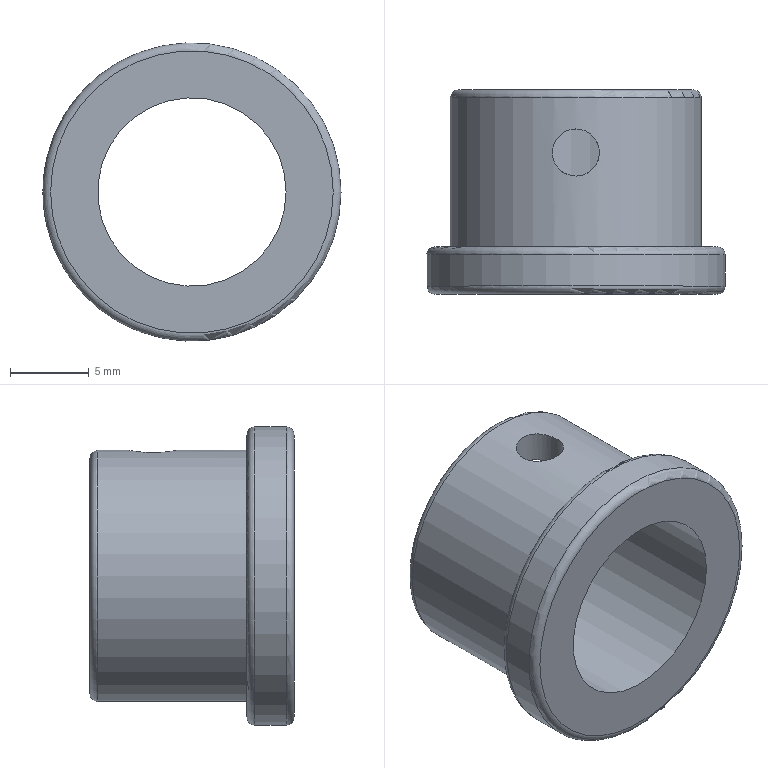Part | STEP file | 1-04.4 | 1 solid | 10 faces | box 19 x 13 x 19 mm | volume 1368 mm3 | cylinder 4 | plane 3 | torus 3 | commonest cylinder face diameters 3 x1 12 x1 16 x1 19 x1
STEP:
#1=CARTESIAN_POINT('',(0.,0.,0.));
#2=DIRECTION('',(0.,0.,1.));
#3=DIRECTION('',(1.,0.,0.));
#4=AXIS2_PLACEMENT_3D('',#1,#2,#3);
#5=CARTESIAN_POINT('',(6.,-3.,0.));
#6=VERTEX_POINT('',#5);
#7=CARTESIAN_POINT('',(6.,10.,0.));
#8=VERTEX_POINT('',#7);
#9=CARTESIAN_POINT('',(6.,-3.,0.));
#10=DIRECTION('',(0.,1.,0.));
#11=VECTOR('',#10,1.);
#12=LINE('',#9,#11);
#13=CARTESIAN_POINT('',(0.,-3.,0.));
#14=DIRECTION('',(0.,1.,0.));
#15=DIRECTION('',(1.,0.,0.));
#16=AXIS2_PLACEMENT_3D('',#13,#14,#15);
#17=CYLINDRICAL_SURFACE('',#16,6.);
#18=CARTESIAN_POINT('',(6.283,0.));
#19=DIRECTION('',(0.,1.));
#20=VECTOR('',#19,1.);
#21=LINE('',#18,#20);
#22=(GEOMETRIC_REPRESENTATION_CONTEXT(2)PARAMETRIC_REPRESENTATION_CONTEXT()REPRESENTATION_CONTEXT('',''));
#23=DEFINITIONAL_REPRESENTATION('',(#21),#22);
#24=PCURVE('',#17,#23);
#25=CARTESIAN_POINT('',(0.,0.));
#26=DIRECTION('',(0.,1.));
#27=VECTOR('',#26,1.);
#28=LINE('',#25,#27);
#29=(GEOMETRIC_REPRESENTATION_CONTEXT(2)PARAMETRIC_REPRESENTATION_CONTEXT()REPRESENTATION_CONTEXT('',''));
#30=DEFINITIONAL_REPRESENTATION('',(#28),#29);
#31=PCURVE('',#17,#30);
#32=SEAM_CURVE('',#12,(#24,#31),.PCURVE_S1.);
#33=EDGE_CURVE('',#6,#8,#32,.T.);
#34=ORIENTED_EDGE('',*,*,#33,.T.);
#35=CARTESIAN_POINT('',(0.,10.,0.));
#36=DIRECTION('',(0.,-1.,0.));
#37=DIRECTION('',(1.,0.,0.));
#38=AXIS2_PLACEMENT_3D('',#35,#36,#37);
#39=CIRCLE('',#38,6.);
#40=CARTESIAN_POINT('',(6.283,13.));
#41=DIRECTION('',(-1.,0.));
#42=VECTOR('',#41,1.);
#43=LINE('',#40,#42);
#44=(GEOMETRIC_REPRESENTATION_CONTEXT(2)PARAMETRIC_REPRESENTATION_CONTEXT()REPRESENTATION_CONTEXT('',''));
#45=DEFINITIONAL_REPRESENTATION('',(#43),#44);
#46=PCURVE('',#17,#45);
#47=CARTESIAN_POINT('',(-2.144,10.,0.));
#48=DIRECTION('',(0.,-1.,0.));
#49=DIRECTION('',(1.,0.,0.));
#50=AXIS2_PLACEMENT_3D('',#47,#48,#49);
#51=PLANE('',#50);
#52=CARTESIAN_POINT('',(2.144,0.));
#53=DIRECTION('',(1.,0.));
#54=AXIS2_PLACEMENT_2D('',#52,#53);
#55=CIRCLE('',#54,6.);
#56=(GEOMETRIC_REPRESENTATION_CONTEXT(2)PARAMETRIC_REPRESENTATION_CONTEXT()REPRESENTATION_CONTEXT('',''));
#57=DEFINITIONAL_REPRESENTATION('',(#55),#56);
#58=PCURVE('',#51,#57);
#59=SURFACE_CURVE('',#39,(#46,#58),.PCURVE_S1.);
#60=EDGE_CURVE('',#8,#8,#59,.T.);
#61=ORIENTED_EDGE('',*,*,#60,.T.);
#62=ORIENTED_EDGE('',*,*,#33,.F.);
#63=CARTESIAN_POINT('',(0.,-3.,0.));
#64=DIRECTION('',(0.,-1.,0.));
#65=DIRECTION('',(1.,0.,0.));
#66=AXIS2_PLACEMENT_3D('',#63,#64,#65);
#67=CIRCLE('',#66,6.);
#68=CARTESIAN_POINT('',(6.283,0.));
#69=DIRECTION('',(-1.,0.));
#70=VECTOR('',#69,1.);
#71=LINE('',#68,#70);
#72=(GEOMETRIC_REPRESENTATION_CONTEXT(2)PARAMETRIC_REPRESENTATION_CONTEXT()REPRESENTATION_CONTEXT('',''));
#73=DEFINITIONAL_REPRESENTATION('',(#71),#72);
#74=PCURVE('',#17,#73);
#75=CARTESIAN_POINT('',(-2.546,-3.,0.));
#76=DIRECTION('',(0.,-1.,0.));
#77=DIRECTION('',(1.,0.,0.));
#78=AXIS2_PLACEMENT_3D('',#75,#76,#77);
#79=PLANE('',#78);
#80=CARTESIAN_POINT('',(2.546,0.));
#81=DIRECTION('',(1.,0.));
#82=AXIS2_PLACEMENT_2D('',#80,#81);
#83=CIRCLE('',#82,6.);
#84=(GEOMETRIC_REPRESENTATION_CONTEXT(2)PARAMETRIC_REPRESENTATION_CONTEXT()REPRESENTATION_CONTEXT('',''));
#85=DEFINITIONAL_REPRESENTATION('',(#83),#84);
#86=PCURVE('',#79,#85);
#87=SURFACE_CURVE('',#67,(#74,#86),.PCURVE_S1.);
#88=EDGE_CURVE('',#6,#6,#87,.T.);
#89=ORIENTED_EDGE('',*,*,#88,.F.);
#90=EDGE_LOOP('',(#34,#61,#62,#89));
#91=FACE_BOUND('',#90,.F.);
#92=CARTESIAN_POINT('',(0.,7.5,6.));
#93=VERTEX_POINT('',#92);
#94=CARTESIAN_POINT('',(0.,7.5,6.));
#95=CARTESIAN_POINT('',(0.2261,7.5,6.));
#96=CARTESIAN_POINT('',(0.9044,7.347,5.962));
#97=CARTESIAN_POINT('',(1.361,6.771,5.844));
#98=CARTESIAN_POINT('',(1.591,5.777,5.787));
#99=CARTESIAN_POINT('',(1.391,5.199,5.854));
#100=CARTESIAN_POINT('',(0.5075,4.478,5.995));
#101=CARTESIAN_POINT('',(-0.09537,4.397,6.022));
#102=CARTESIAN_POINT('',(-1.153,4.875,5.913));
#103=CARTESIAN_POINT('',(-1.5,5.408,5.809));
#104=CARTESIAN_POINT('',(-1.5,6.74,5.809));
#105=CARTESIAN_POINT('',(-0.9622,7.368,5.967));
#106=CARTESIAN_POINT('',(-0.18,7.49,5.998));
#107=CARTESIAN_POINT('',(-0.1029,7.498,6.));
#108=CARTESIAN_POINT('',(-0.02572,7.5,6.));
#109=CARTESIAN_POINT('',(0.,7.5,6.));
#110=B_SPLINE_CURVE_WITH_KNOTS('',3,(#94,#95,#96,#97,#98,#99,#100,#101,#102,#103,#104,#105,#106,#107,#108,#109),.UNSPECIFIED.,.T.,.F.,(1,3,1,2,2,2,2,2,1,3,1),(-0.03834,0.,0.3333,1.,1.864,2.726,3.611,4.715,4.792,4.83,5.163),.UNSPECIFIED.);
#111=CARTESIAN_POINT('',(4.712,10.5));
#112=CARTESIAN_POINT('',(4.725,10.5));
#113=CARTESIAN_POINT('',(4.75,10.489));
#114=CARTESIAN_POINT('',(4.786,10.44));
#115=CARTESIAN_POINT('',(4.821,10.359));
#116=CARTESIAN_POINT('',(4.853,10.248));
#117=CARTESIAN_POINT('',(4.882,10.11));
#118=CARTESIAN_POINT('',(4.908,9.949));
#119=CARTESIAN_POINT('',(4.929,9.768));
#120=CARTESIAN_POINT('',(4.946,9.572));
#121=CARTESIAN_POINT('',(4.958,9.362));
#122=CARTESIAN_POINT('',(4.965,9.147));
#123=CARTESIAN_POINT('',(4.966,8.934));
#124=CARTESIAN_POINT('',(4.961,8.724));
#125=CARTESIAN_POINT('',(4.952,8.52));
#126=CARTESIAN_POINT('',(4.939,8.327));
#127=CARTESIAN_POINT('',(4.92,8.145));
#128=CARTESIAN_POINT('',(4.898,7.98));
#129=CARTESIAN_POINT('',(4.871,7.831));
#130=CARTESIAN_POINT('',(4.841,7.707));
#131=CARTESIAN_POINT('',(4.81,7.612));
#132=CARTESIAN_POINT('',(4.776,7.544));
#133=CARTESIAN_POINT('',(4.742,7.505));
#134=CARTESIAN_POINT('',(4.707,7.495));
#135=CARTESIAN_POINT('',(4.672,7.514));
#136=CARTESIAN_POINT('',(4.638,7.563));
#137=CARTESIAN_POINT('',(4.603,7.643));
#138=CARTESIAN_POINT('',(4.572,7.751));
#139=CARTESIAN_POINT('',(4.544,7.883));
#140=CARTESIAN_POINT('',(4.519,8.035));
#141=CARTESIAN_POINT('',(4.498,8.207));
#142=CARTESIAN_POINT('',(4.481,8.394));
#143=CARTESIAN_POINT('',(4.468,8.594));
#144=CARTESIAN_POINT('',(4.461,8.804));
#145=CARTESIAN_POINT('',(4.459,9.024));
#146=CARTESIAN_POINT('',(4.462,9.241));
#147=CARTESIAN_POINT('',(4.471,9.448));
#148=CARTESIAN_POINT('',(4.484,9.644));
#149=CARTESIAN_POINT('',(4.501,9.826));
#150=CARTESIAN_POINT('',(4.523,9.991));
#151=CARTESIAN_POINT('',(4.547,10.138));
#152=CARTESIAN_POINT('',(4.576,10.263));
#153=CARTESIAN_POINT('',(4.606,10.365));
#154=CARTESIAN_POINT('',(4.64,10.441));
#155=CARTESIAN_POINT('',(4.675,10.489));
#156=CARTESIAN_POINT('',(4.7,10.5));
#157=CARTESIAN_POINT('',(4.712,10.5));
#158=B_SPLINE_CURVE_WITH_KNOTS('',3,(#111,#112,#113,#114,#115,#116,#117,#118,#119,#120,#121,#122,#123,#124,#125,#126,#127,#128,#129,#130,#131,#132,#133,#134,#135,#136,#137,#138,#139,#140,#141,#142,#143,#144,#145,#146,#147,#148,#149,#150,#151,#152,#153,#154,#155,#156,#157),.UNSPECIFIED.,.T.,.F.,(4,1,1,1,1,1,1,1,1,1,1,1,1,1,1,1,1,1,1,1,1,1,1,1,1,1,1,1,1,1,1,1,1,1,1,1,1,1,1,1,1,1,1,1,4),(0.,0.1098,0.2195,0.3293,0.4391,0.5489,0.6586,0.7684,0.8782,0.9879,1.098,1.207,1.317,1.427,1.537,1.647,1.756,1.866,1.976,2.086,2.195,2.305,2.415,2.525,2.634,2.744,2.854,2.964,3.074,3.183,3.293,3.403,3.513,3.622,3.732,3.842,3.952,4.062,4.171,4.281,4.391,4.501,4.61,4.72,4.83),.QUASI_UNIFORM_KNOTS.);
#159=(GEOMETRIC_REPRESENTATION_CONTEXT(2)PARAMETRIC_REPRESENTATION_CONTEXT()REPRESENTATION_CONTEXT('',''));
#160=DEFINITIONAL_REPRESENTATION('',(#158),#159);
#161=PCURVE('',#17,#160);
#162=CARTESIAN_POINT('',(0.,6.,0.));
#163=DIRECTION('',(0.,0.,1.));
#164=DIRECTION('',(0.,1.,0.));
#165=AXIS2_PLACEMENT_3D('',#162,#163,#164);
#166=CYLINDRICAL_SURFACE('',#165,1.5);
#167=CARTESIAN_POINT('',(6.283,6.));
#168=CARTESIAN_POINT('',(6.234,6.));
#169=CARTESIAN_POINT('',(6.134,5.997));
#170=CARTESIAN_POINT('',(5.986,5.986));
#171=CARTESIAN_POINT('',(5.838,5.967));
#172=CARTESIAN_POINT('',(5.691,5.943));
#173=CARTESIAN_POINT('',(5.543,5.916));
#174=CARTESIAN_POINT('',(5.396,5.888));
#175=CARTESIAN_POINT('',(5.249,5.86));
#176=CARTESIAN_POINT('',(5.102,5.837));
#177=CARTESIAN_POINT('',(4.956,5.819));
#178=CARTESIAN_POINT('',(4.81,5.81));
#179=CARTESIAN_POINT('',(4.668,5.811));
#180=CARTESIAN_POINT('',(4.528,5.818));
#181=CARTESIAN_POINT('',(4.388,5.832));
#182=CARTESIAN_POINT('',(4.249,5.85));
#183=CARTESIAN_POINT('',(4.109,5.873));
#184=CARTESIAN_POINT('',(3.968,5.898));
#185=CARTESIAN_POINT('',(3.823,5.925));
#186=CARTESIAN_POINT('',(3.68,5.951));
#187=CARTESIAN_POINT('',(3.539,5.971));
#188=CARTESIAN_POINT('',(3.399,5.985));
#189=CARTESIAN_POINT('',(3.26,5.995));
#190=CARTESIAN_POINT('',(3.121,5.998));
#191=CARTESIAN_POINT('',(2.98,5.994));
#192=CARTESIAN_POINT('',(2.839,5.984));
#193=CARTESIAN_POINT('',(2.693,5.966));
#194=CARTESIAN_POINT('',(2.549,5.942));
#195=CARTESIAN_POINT('',(2.407,5.916));
#196=CARTESIAN_POINT('',(2.266,5.89));
#197=CARTESIAN_POINT('',(2.126,5.864));
#198=CARTESIAN_POINT('',(1.986,5.842));
#199=CARTESIAN_POINT('',(1.844,5.824));
#200=CARTESIAN_POINT('',(1.701,5.812));
#201=CARTESIAN_POINT('',(1.555,5.808));
#202=CARTESIAN_POINT('',(1.41,5.814));
#203=CARTESIAN_POINT('',(1.268,5.827));
#204=CARTESIAN_POINT('',(1.129,5.846));
#205=CARTESIAN_POINT('',(0.9901,5.868));
#206=CARTESIAN_POINT('',(0.852,5.894));
#207=CARTESIAN_POINT('',(0.7139,5.92));
#208=CARTESIAN_POINT('',(0.5752,5.945));
#209=CARTESIAN_POINT('',(0.4353,5.967));
#210=CARTESIAN_POINT('',(0.2934,5.985));
#211=CARTESIAN_POINT('',(0.1477,5.997));
#212=CARTESIAN_POINT('',(0.04935,6.));
#213=CARTESIAN_POINT('',(0.,6.));
#214=B_SPLINE_CURVE_WITH_KNOTS('',3,(#167,#168,#169,#170,#171,#172,#173,#174,#175,#176,#177,#178,#179,#180,#181,#182,#183,#184,#185,#186,#187,#188,#189,#190,#191,#192,#193,#194,#195,#196,#197,#198,#199,#200,#201,#202,#203,#204,#205,#206,#207,#208,#209,#210,#211,#212,#213),.UNSPECIFIED.,.F.,.F.,(4,1,1,1,1,1,1,1,1,1,1,1,1,1,1,1,1,1,1,1,1,1,1,1,1,1,1,1,1,1,1,1,1,1,1,1,1,1,1,1,1,1,1,1,4),(0.,0.1098,0.2195,0.3293,0.4391,0.5489,0.6586,0.7684,0.8782,0.9879,1.098,1.207,1.317,1.427,1.537,1.647,1.756,1.866,1.976,2.086,2.195,2.305,2.415,2.525,2.634,2.744,2.854,2.964,3.074,3.183,3.293,3.403,3.513,3.622,3.732,3.842,3.952,4.062,4.171,4.281,4.391,4.501,4.61,4.72,4.83),.QUASI_UNIFORM_KNOTS.);
#215=(GEOMETRIC_REPRESENTATION_CONTEXT(2)PARAMETRIC_REPRESENTATION_CONTEXT()REPRESENTATION_CONTEXT('',''));
#216=DEFINITIONAL_REPRESENTATION('',(#214),#215);
#217=PCURVE('',#166,#216);
#218=SURFACE_CURVE('',#110,(#161,#217),.PCURVE_S1.);
#219=EDGE_CURVE('',#93,#93,#218,.T.);
#220=ORIENTED_EDGE('',*,*,#219,.T.);
#221=EDGE_LOOP('',(#220));
#222=FACE_BOUND('',#221,.F.);
#223=ADVANCED_FACE('',(#91,#222),#17,.F.);
#224=CARTESIAN_POINT('',(0.,7.5,8.));
#225=VERTEX_POINT('',#224);
#226=CARTESIAN_POINT('',(0.,7.5,6.));
#227=DIRECTION('',(0.,0.,1.));
#228=VECTOR('',#227,1.);
#229=LINE('',#226,#228);
#230=CARTESIAN_POINT('',(0.,6.));
#231=DIRECTION('',(0.,1.));
#232=VECTOR('',#231,1.);
#233=LINE('',#230,#232);
#234=(GEOMETRIC_REPRESENTATION_CONTEXT(2)PARAMETRIC_REPRESENTATION_CONTEXT()REPRESENTATION_CONTEXT('',''));
#235=DEFINITIONAL_REPRESENTATION('',(#233),#234);
#236=PCURVE('',#166,#235);
#237=CARTESIAN_POINT('',(6.283,6.));
#238=DIRECTION('',(0.,1.));
#239=VECTOR('',#238,1.);
#240=LINE('',#237,#239);
#241=(GEOMETRIC_REPRESENTATION_CONTEXT(2)PARAMETRIC_REPRESENTATION_CONTEXT()REPRESENTATION_CONTEXT('',''));
#242=DEFINITIONAL_REPRESENTATION('',(#240),#241);
#243=PCURVE('',#166,#242);
#244=SEAM_CURVE('',#229,(#236,#243),.PCURVE_S1.);
#245=EDGE_CURVE('',#93,#225,#244,.T.);
#246=ORIENTED_EDGE('',*,*,#245,.F.);
#247=ORIENTED_EDGE('',*,*,#219,.F.);
#248=ORIENTED_EDGE('',*,*,#245,.T.);
#249=CARTESIAN_POINT('',(0.,7.5,8.));
#250=CARTESIAN_POINT('',(-0.03438,7.5,8.));
#251=CARTESIAN_POINT('',(-0.1375,7.496,7.999));
#252=CARTESIAN_POINT('',(-0.2404,7.482,7.997));
#253=CARTESIAN_POINT('',(-1.002,7.323,7.967));
#254=CARTESIAN_POINT('',(-1.5,6.712,7.858));
#255=CARTESIAN_POINT('',(-1.5,5.288,7.858));
#256=CARTESIAN_POINT('',(-1.002,4.677,7.967));
#257=CARTESIAN_POINT('',(0.7679,4.306,8.035));
#258=CARTESIAN_POINT('',(1.71,5.272,7.819));
#259=CARTESIAN_POINT('',(1.36,6.774,7.884));
#260=CARTESIAN_POINT('',(0.9023,7.347,7.971));
#261=CARTESIAN_POINT('',(0.2256,7.5,8.));
#262=CARTESIAN_POINT('',(0.,7.5,8.));
#263=B_SPLINE_CURVE_WITH_KNOTS('',3,(#249,#250,#251,#252,#253,#254,#255,#256,#257,#258,#259,#260,#261,#262),.UNSPECIFIED.,.T.,.F.,(1,3,1,2,2,2,2,1,3,1),(-0.3333,0.,0.05142,0.1542,1.216,2.277,3.922,4.589,4.922,4.974),.UNSPECIFIED.);
#264=CARTESIAN_POINT('',(0.,8.));
#265=CARTESIAN_POINT('',(0.04988,8.));
#266=CARTESIAN_POINT('',(0.15,7.998));
#267=CARTESIAN_POINT('',(0.2994,7.989));
#268=CARTESIAN_POINT('',(0.4446,7.975));
#269=CARTESIAN_POINT('',(0.5878,7.957));
#270=CARTESIAN_POINT('',(0.7296,7.938));
#271=CARTESIAN_POINT('',(0.8708,7.918));
#272=CARTESIAN_POINT('',(1.012,7.899));
#273=CARTESIAN_POINT('',(1.154,7.882));
#274=CARTESIAN_POINT('',(1.297,7.869));
#275=CARTESIAN_POINT('',(1.441,7.86));
#276=CARTESIAN_POINT('',(1.591,7.857));
#277=CARTESIAN_POINT('',(1.739,7.861));
#278=CARTESIAN_POINT('',(1.883,7.872));
#279=CARTESIAN_POINT('',(2.025,7.886));
#280=CARTESIAN_POINT('',(2.167,7.904));
#281=CARTESIAN_POINT('',(2.308,7.924));
#282=CARTESIAN_POINT('',(2.449,7.943));
#283=CARTESIAN_POINT('',(2.591,7.962));
#284=CARTESIAN_POINT('',(2.735,7.979));
#285=CARTESIAN_POINT('',(2.881,7.992));
#286=CARTESIAN_POINT('',(3.031,7.999));
#287=CARTESIAN_POINT('',(3.173,8.));
#288=CARTESIAN_POINT('',(3.311,7.995));
#289=CARTESIAN_POINT('',(3.447,7.986));
#290=CARTESIAN_POINT('',(3.58,7.973));
#291=CARTESIAN_POINT('',(3.713,7.958));
#292=CARTESIAN_POINT('',(3.845,7.941));
#293=CARTESIAN_POINT('',(3.977,7.923));
#294=CARTESIAN_POINT('',(4.109,7.905));
#295=CARTESIAN_POINT('',(4.241,7.889));
#296=CARTESIAN_POINT('',(4.374,7.876));
#297=CARTESIAN_POINT('',(4.508,7.865));
#298=CARTESIAN_POINT('',(4.645,7.859));
#299=CARTESIAN_POINT('',(4.786,7.858));
#300=CARTESIAN_POINT('',(4.932,7.864));
#301=CARTESIAN_POINT('',(5.082,7.876));
#302=CARTESIAN_POINT('',(5.231,7.894));
#303=CARTESIAN_POINT('',(5.381,7.914));
#304=CARTESIAN_POINT('',(5.531,7.935));
#305=CARTESIAN_POINT('',(5.681,7.956));
#306=CARTESIAN_POINT('',(5.83,7.975));
#307=CARTESIAN_POINT('',(5.981,7.989));
#308=CARTESIAN_POINT('',(6.132,7.998));
#309=CARTESIAN_POINT('',(6.233,8.));
#310=CARTESIAN_POINT('',(6.283,8.));
#311=B_SPLINE_CURVE_WITH_KNOTS('',3,(#264,#265,#266,#267,#268,#269,#270,#271,#272,#273,#274,#275,#276,#277,#278,#279,#280,#281,#282,#283,#284,#285,#286,#287,#288,#289,#290,#291,#292,#293,#294,#295,#296,#297,#298,#299,#300,#301,#302,#303,#304,#305,#306,#307,#308,#309,#310),.UNSPECIFIED.,.F.,.F.,(4,1,1,1,1,1,1,1,1,1,1,1,1,1,1,1,1,1,1,1,1,1,1,1,1,1,1,1,1,1,1,1,1,1,1,1,1,1,1,1,1,1,1,1,4),(0.,0.1119,0.2237,0.3356,0.4475,0.5593,0.6712,0.7831,0.8949,1.007,1.119,1.231,1.342,1.454,1.566,1.678,1.79,1.902,2.014,2.125,2.237,2.349,2.461,2.573,2.685,2.797,2.909,3.02,3.132,3.244,3.356,3.468,3.58,3.692,3.803,3.915,4.027,4.139,4.251,4.363,4.475,4.587,4.698,4.81,4.922),.QUASI_UNIFORM_KNOTS.);
#312=(GEOMETRIC_REPRESENTATION_CONTEXT(2)PARAMETRIC_REPRESENTATION_CONTEXT()REPRESENTATION_CONTEXT('',''));
#313=DEFINITIONAL_REPRESENTATION('',(#311),#312);
#314=PCURVE('',#166,#313);
#315=CARTESIAN_POINT('',(0.,0.,0.));
#316=DIRECTION('',(0.,1.,0.));
#317=DIRECTION('',(1.,0.,0.));
#318=AXIS2_PLACEMENT_3D('',#315,#316,#317);
#319=CYLINDRICAL_SURFACE('',#318,8.);
#320=CARTESIAN_POINT('',(4.712,7.5));
#321=CARTESIAN_POINT('',(4.703,7.5));
#322=CARTESIAN_POINT('',(4.684,7.489));
#323=CARTESIAN_POINT('',(4.657,7.439));
#324=CARTESIAN_POINT('',(4.631,7.359));
#325=CARTESIAN_POINT('',(4.608,7.253));
#326=CARTESIAN_POINT('',(4.587,7.122));
#327=CARTESIAN_POINT('',(4.568,6.97));
#328=CARTESIAN_POINT('',(4.552,6.798));
#329=CARTESIAN_POINT('',(4.54,6.61));
#330=CARTESIAN_POINT('',(4.53,6.408));
#331=CARTESIAN_POINT('',(4.525,6.194));
#332=CARTESIAN_POINT('',(4.523,5.97));
#333=CARTESIAN_POINT('',(4.526,5.749));
#334=CARTESIAN_POINT('',(4.532,5.538));
#335=CARTESIAN_POINT('',(4.543,5.339));
#336=CARTESIAN_POINT('',(4.556,5.155));
#337=CARTESIAN_POINT('',(4.573,4.988));
#338=CARTESIAN_POINT('',(4.592,4.841));
#339=CARTESIAN_POINT('',(4.614,4.717));
#340=CARTESIAN_POINT('',(4.638,4.617));
#341=CARTESIAN_POINT('',(4.664,4.545));
#342=CARTESIAN_POINT('',(4.692,4.504));
#343=CARTESIAN_POINT('',(4.718,4.494));
#344=CARTESIAN_POINT('',(4.744,4.515));
#345=CARTESIAN_POINT('',(4.769,4.563));
#346=CARTESIAN_POINT('',(4.792,4.636));
#347=CARTESIAN_POINT('',(4.814,4.733));
#348=CARTESIAN_POINT('',(4.834,4.852));
#349=CARTESIAN_POINT('',(4.852,4.99));
#350=CARTESIAN_POINT('',(4.868,5.145));
#351=CARTESIAN_POINT('',(4.881,5.316));
#352=CARTESIAN_POINT('',(4.891,5.5));
#353=CARTESIAN_POINT('',(4.898,5.695));
#354=CARTESIAN_POINT('',(4.901,5.899));
#355=CARTESIAN_POINT('',(4.901,6.11));
#356=CARTESIAN_POINT('',(4.897,6.327));
#357=CARTESIAN_POINT('',(4.889,6.543));
#358=CARTESIAN_POINT('',(4.876,6.745));
#359=CARTESIAN_POINT('',(4.86,6.931));
#360=CARTESIAN_POINT('',(4.841,7.098));
#361=CARTESIAN_POINT('',(4.819,7.24));
#362=CARTESIAN_POINT('',(4.795,7.355));
#363=CARTESIAN_POINT('',(4.768,7.438));
#364=CARTESIAN_POINT('',(4.741,7.489));
#365=CARTESIAN_POINT('',(4.722,7.5));
#366=CARTESIAN_POINT('',(4.712,7.5));
#367=B_SPLINE_CURVE_WITH_KNOTS('',3,(#320,#321,#322,#323,#324,#325,#326,#327,#328,#329,#330,#331,#332,#333,#334,#335,#336,#337,#338,#339,#340,#341,#342,#343,#344,#345,#346,#347,#348,#349,#350,#351,#352,#353,#354,#355,#356,#357,#358,#359,#360,#361,#362,#363,#364,#365,#366),.UNSPECIFIED.,.T.,.F.,(4,1,1,1,1,1,1,1,1,1,1,1,1,1,1,1,1,1,1,1,1,1,1,1,1,1,1,1,1,1,1,1,1,1,1,1,1,1,1,1,1,1,1,1,4),(0.,0.1119,0.2237,0.3356,0.4475,0.5593,0.6712,0.7831,0.8949,1.007,1.119,1.231,1.342,1.454,1.566,1.678,1.79,1.902,2.014,2.125,2.237,2.349,2.461,2.573,2.685,2.797,2.909,3.02,3.132,3.244,3.356,3.468,3.58,3.692,3.803,3.915,4.027,4.139,4.251,4.363,4.475,4.587,4.698,4.81,4.922),.QUASI_UNIFORM_KNOTS.);
#368=(GEOMETRIC_REPRESENTATION_CONTEXT(2)PARAMETRIC_REPRESENTATION_CONTEXT()REPRESENTATION_CONTEXT('',''));
#369=DEFINITIONAL_REPRESENTATION('',(#367),#368);
#370=PCURVE('',#319,#369);
#371=SURFACE_CURVE('',#263,(#314,#370),.PCURVE_S1.);
#372=EDGE_CURVE('',#225,#225,#371,.T.);
#373=ORIENTED_EDGE('',*,*,#372,.F.);
#374=EDGE_LOOP('',(#246,#247,#248,#373));
#375=FACE_BOUND('',#374,.F.);
#376=ADVANCED_FACE('',(#375),#166,.F.);
#377=CARTESIAN_POINT('',(9.,0.,0.));
#378=VERTEX_POINT('',#377);
#379=CARTESIAN_POINT('',(0.,0.,0.));
#380=DIRECTION('',(0.,1.,0.));
#381=DIRECTION('',(1.,0.,0.));
#382=AXIS2_PLACEMENT_3D('',#379,#380,#381);
#383=CIRCLE('',#382,9.);
#384=CARTESIAN_POINT('',(-2.546,0.,0.));
#385=DIRECTION('',(0.,-1.,0.));
#386=DIRECTION('',(1.,0.,0.));
#387=AXIS2_PLACEMENT_3D('',#384,#385,#386);
#388=PLANE('',#387);
#389=CARTESIAN_POINT('',(11.546,0.));
#390=CARTESIAN_POINT('',(11.546,-15.588));
#391=CARTESIAN_POINT('',(-1.954,-7.794));
#392=CARTESIAN_POINT('',(-15.454,0.));
#393=CARTESIAN_POINT('',(-1.954,7.794));
#394=CARTESIAN_POINT('',(11.546,15.588));
#395=CARTESIAN_POINT('',(11.546,0.));
#396=(BOUNDED_CURVE()B_SPLINE_CURVE(2,(#389,#390,#391,#392,#393,#394,#395),.UNSPECIFIED.,.T.,.F.)B_SPLINE_CURVE_WITH_KNOTS((1,2,2,2,2,1),(-2.094,0.,2.094,4.189,6.283,8.378),.UNSPECIFIED.)CURVE()GEOMETRIC_REPRESENTATION_ITEM()RATIONAL_B_SPLINE_CURVE((1.,0.5,1.,0.5,1.,0.5,1.))REPRESENTATION_ITEM(''));
#397=(GEOMETRIC_REPRESENTATION_CONTEXT(2)PARAMETRIC_REPRESENTATION_CONTEXT()REPRESENTATION_CONTEXT('',''));
#398=DEFINITIONAL_REPRESENTATION('',(#396),#397);
#399=PCURVE('',#388,#398);
#400=CARTESIAN_POINT('',(0.,-0.5,0.));
#401=DIRECTION('',(0.,-1.,0.));
#402=DIRECTION('',(1.,0.,0.));
#403=AXIS2_PLACEMENT_3D('',#400,#401,#402);
#404=TOROIDAL_SURFACE('',#403,9.,0.5);
#405=CARTESIAN_POINT('',(6.283,4.712));
#406=DIRECTION('',(-1.,0.));
#407=VECTOR('',#406,1.);
#408=LINE('',#405,#407);
#409=(GEOMETRIC_REPRESENTATION_CONTEXT(2)PARAMETRIC_REPRESENTATION_CONTEXT()REPRESENTATION_CONTEXT('',''));
#410=DEFINITIONAL_REPRESENTATION('',(#408),#409);
#411=PCURVE('',#404,#410);
#412=SURFACE_CURVE('',#383,(#399,#411),.PCURVE_S1.);
#413=EDGE_CURVE('',#378,#378,#412,.T.);
#414=ORIENTED_EDGE('',*,*,#413,.F.);
#415=EDGE_LOOP('',(#414));
#416=FACE_BOUND('',#415,.F.);
#417=CARTESIAN_POINT('',(8.,0.,0.));
#418=VERTEX_POINT('',#417);
#419=CARTESIAN_POINT('',(0.,0.,0.));
#420=DIRECTION('',(0.,-1.,0.));
#421=DIRECTION('',(1.,0.,0.));
#422=AXIS2_PLACEMENT_3D('',#419,#420,#421);
#423=CIRCLE('',#422,8.);
#424=CARTESIAN_POINT('',(2.546,0.));
#425=DIRECTION('',(1.,0.));
#426=AXIS2_PLACEMENT_2D('',#424,#425);
#427=CIRCLE('',#426,8.);
#428=(GEOMETRIC_REPRESENTATION_CONTEXT(2)PARAMETRIC_REPRESENTATION_CONTEXT()REPRESENTATION_CONTEXT('',''));
#429=DEFINITIONAL_REPRESENTATION('',(#427),#428);
#430=PCURVE('',#388,#429);
#431=CARTESIAN_POINT('',(6.283,0.));
#432=DIRECTION('',(-1.,0.));
#433=VECTOR('',#432,1.);
#434=LINE('',#431,#433);
#435=(GEOMETRIC_REPRESENTATION_CONTEXT(2)PARAMETRIC_REPRESENTATION_CONTEXT()REPRESENTATION_CONTEXT('',''));
#436=DEFINITIONAL_REPRESENTATION('',(#434),#435);
#437=PCURVE('',#319,#436);
#438=SURFACE_CURVE('',#423,(#430,#437),.PCURVE_S1.);
#439=EDGE_CURVE('',#418,#418,#438,.T.);
#440=ORIENTED_EDGE('',*,*,#439,.F.);
#441=EDGE_LOOP('',(#440));
#442=FACE_BOUND('',#441,.F.);
#443=ADVANCED_FACE('',(#416,#442),#388,.F.);
#444=CARTESIAN_POINT('',(9.5,-0.5,0.));
#445=VERTEX_POINT('',#444);
#446=CARTESIAN_POINT('',(9.5,-2.5,0.));
#447=VERTEX_POINT('',#446);
#448=CARTESIAN_POINT('',(9.5,-0.5,0.));
#449=DIRECTION('',(0.,-1.,0.));
#450=VECTOR('',#449,1.);
#451=LINE('',#448,#450);
#452=CARTESIAN_POINT('',(0.,0.,0.));
#453=DIRECTION('',(0.,-1.,0.));
#454=DIRECTION('',(1.,0.,0.));
#455=AXIS2_PLACEMENT_3D('',#452,#453,#454);
#456=CYLINDRICAL_SURFACE('',#455,9.5);
#457=CARTESIAN_POINT('',(6.283,0.5));
#458=DIRECTION('',(0.,1.));
#459=VECTOR('',#458,1.);
#460=LINE('',#457,#459);
#461=(GEOMETRIC_REPRESENTATION_CONTEXT(2)PARAMETRIC_REPRESENTATION_CONTEXT()REPRESENTATION_CONTEXT('',''));
#462=DEFINITIONAL_REPRESENTATION('',(#460),#461);
#463=PCURVE('',#456,#462);
#464=CARTESIAN_POINT('',(0.,0.5));
#465=DIRECTION('',(0.,1.));
#466=VECTOR('',#465,1.);
#467=LINE('',#464,#466);
#468=(GEOMETRIC_REPRESENTATION_CONTEXT(2)PARAMETRIC_REPRESENTATION_CONTEXT()REPRESENTATION_CONTEXT('',''));
#469=DEFINITIONAL_REPRESENTATION('',(#467),#468);
#470=PCURVE('',#456,#469);
#471=SEAM_CURVE('',#451,(#463,#470),.PCURVE_S1.);
#472=EDGE_CURVE('',#445,#447,#471,.T.);
#473=ORIENTED_EDGE('',*,*,#472,.T.);
#474=CARTESIAN_POINT('',(0.,-2.5,0.));
#475=DIRECTION('',(0.,1.,0.));
#476=DIRECTION('',(1.,0.,0.));
#477=AXIS2_PLACEMENT_3D('',#474,#475,#476);
#478=CIRCLE('',#477,9.5);
#479=CARTESIAN_POINT('',(6.283,2.5));
#480=DIRECTION('',(-1.,0.));
#481=VECTOR('',#480,1.);
#482=LINE('',#479,#481);
#483=(GEOMETRIC_REPRESENTATION_CONTEXT(2)PARAMETRIC_REPRESENTATION_CONTEXT()REPRESENTATION_CONTEXT('',''));
#484=DEFINITIONAL_REPRESENTATION('',(#482),#483);
#485=PCURVE('',#456,#484);
#486=CARTESIAN_POINT('',(0.,-2.5,0.));
#487=DIRECTION('',(0.,-1.,0.));
#488=DIRECTION('',(1.,0.,0.));
#489=AXIS2_PLACEMENT_3D('',#486,#487,#488);
#490=TOROIDAL_SURFACE('',#489,9.,0.5);
#491=CARTESIAN_POINT('',(6.283,0.));
#492=DIRECTION('',(-1.,0.));
#493=VECTOR('',#492,1.);
#494=LINE('',#491,#493);
#495=(GEOMETRIC_REPRESENTATION_CONTEXT(2)PARAMETRIC_REPRESENTATION_CONTEXT()REPRESENTATION_CONTEXT('',''));
#496=DEFINITIONAL_REPRESENTATION('',(#494),#495);
#497=PCURVE('',#490,#496);
#498=SURFACE_CURVE('',#478,(#485,#497),.PCURVE_S1.);
#499=EDGE_CURVE('',#447,#447,#498,.T.);
#500=ORIENTED_EDGE('',*,*,#499,.T.);
#501=ORIENTED_EDGE('',*,*,#472,.F.);
#502=CARTESIAN_POINT('',(0.,-0.5,0.));
#503=DIRECTION('',(0.,1.,0.));
#504=DIRECTION('',(1.,0.,0.));
#505=AXIS2_PLACEMENT_3D('',#502,#503,#504);
#506=CIRCLE('',#505,9.5);
#507=CARTESIAN_POINT('',(6.283,0.5));
#508=DIRECTION('',(-1.,0.));
#509=VECTOR('',#508,1.);
#510=LINE('',#507,#509);
#511=(GEOMETRIC_REPRESENTATION_CONTEXT(2)PARAMETRIC_REPRESENTATION_CONTEXT()REPRESENTATION_CONTEXT('',''));
#512=DEFINITIONAL_REPRESENTATION('',(#510),#511);
#513=PCURVE('',#456,#512);
#514=CARTESIAN_POINT('',(6.283,6.283));
#515=DIRECTION('',(-1.,0.));
#516=VECTOR('',#515,1.);
#517=LINE('',#514,#516);
#518=(GEOMETRIC_REPRESENTATION_CONTEXT(2)PARAMETRIC_REPRESENTATION_CONTEXT()REPRESENTATION_CONTEXT('',''));
#519=DEFINITIONAL_REPRESENTATION('',(#517),#518);
#520=PCURVE('',#404,#519);
#521=SURFACE_CURVE('',#506,(#513,#520),.PCURVE_S1.);
#522=EDGE_CURVE('',#445,#445,#521,.T.);
#523=ORIENTED_EDGE('',*,*,#522,.F.);
#524=EDGE_LOOP('',(#473,#500,#501,#523));
#525=FACE_BOUND('',#524,.T.);
#526=ADVANCED_FACE('',(#525),#456,.T.);
#527=CARTESIAN_POINT('',(7.5,10.,0.));
#528=VERTEX_POINT('',#527);
#529=CARTESIAN_POINT('',(0.,10.,0.));
#530=DIRECTION('',(0.,-1.,0.));
#531=DIRECTION('',(1.,0.,0.));
#532=AXIS2_PLACEMENT_3D('',#529,#530,#531);
#533=CIRCLE('',#532,7.5);
#534=CARTESIAN_POINT('',(2.144,0.));
#535=DIRECTION('',(1.,0.));
#536=AXIS2_PLACEMENT_2D('',#534,#535);
#537=CIRCLE('',#536,7.5);
#538=(GEOMETRIC_REPRESENTATION_CONTEXT(2)PARAMETRIC_REPRESENTATION_CONTEXT()REPRESENTATION_CONTEXT('',''));
#539=DEFINITIONAL_REPRESENTATION('',(#537),#538);
#540=PCURVE('',#51,#539);
#541=CARTESIAN_POINT('',(0.,9.5,0.));
#542=DIRECTION('',(0.,1.,0.));
#543=DIRECTION('',(1.,0.,0.));
#544=AXIS2_PLACEMENT_3D('',#541,#542,#543);
#545=TOROIDAL_SURFACE('',#544,7.5,0.5);
#546=CARTESIAN_POINT('',(6.283,1.571));
#547=DIRECTION('',(-1.,0.));
#548=VECTOR('',#547,1.);
#549=LINE('',#546,#548);
#550=(GEOMETRIC_REPRESENTATION_CONTEXT(2)PARAMETRIC_REPRESENTATION_CONTEXT()REPRESENTATION_CONTEXT('',''));
#551=DEFINITIONAL_REPRESENTATION('',(#549),#550);
#552=PCURVE('',#545,#551);
#553=SURFACE_CURVE('',#533,(#540,#552),.PCURVE_S1.);
#554=EDGE_CURVE('',#528,#528,#553,.T.);
#555=ORIENTED_EDGE('',*,*,#554,.T.);
#556=EDGE_LOOP('',(#555));
#557=FACE_BOUND('',#556,.F.);
#558=ORIENTED_EDGE('',*,*,#60,.F.);
#559=EDGE_LOOP('',(#558));
#560=FACE_BOUND('',#559,.F.);
#561=ADVANCED_FACE('',(#557,#560),#51,.F.);
#562=CARTESIAN_POINT('',(9.,-3.,0.));
#563=VERTEX_POINT('',#562);
#564=CARTESIAN_POINT('',(0.,-3.,0.));
#565=DIRECTION('',(0.,1.,0.));
#566=DIRECTION('',(1.,0.,0.));
#567=AXIS2_PLACEMENT_3D('',#564,#565,#566);
#568=CIRCLE('',#567,9.);
#569=CARTESIAN_POINT('',(11.546,0.));
#570=CARTESIAN_POINT('',(11.546,-15.588));
#571=CARTESIAN_POINT('',(-1.954,-7.794));
#572=CARTESIAN_POINT('',(-15.454,0.));
#573=CARTESIAN_POINT('',(-1.954,7.794));
#574=CARTESIAN_POINT('',(11.546,15.588));
#575=CARTESIAN_POINT('',(11.546,0.));
#576=(BOUNDED_CURVE()B_SPLINE_CURVE(2,(#569,#570,#571,#572,#573,#574,#575),.UNSPECIFIED.,.T.,.F.)B_SPLINE_CURVE_WITH_KNOTS((1,2,2,2,2,1),(-2.094,0.,2.094,4.189,6.283,8.378),.UNSPECIFIED.)CURVE()GEOMETRIC_REPRESENTATION_ITEM()RATIONAL_B_SPLINE_CURVE((1.,0.5,1.,0.5,1.,0.5,1.))REPRESENTATION_ITEM(''));
#577=(GEOMETRIC_REPRESENTATION_CONTEXT(2)PARAMETRIC_REPRESENTATION_CONTEXT()REPRESENTATION_CONTEXT('',''));
#578=DEFINITIONAL_REPRESENTATION('',(#576),#577);
#579=PCURVE('',#79,#578);
#580=CARTESIAN_POINT('',(6.283,1.571));
#581=DIRECTION('',(-1.,0.));
#582=VECTOR('',#581,1.);
#583=LINE('',#580,#582);
#584=(GEOMETRIC_REPRESENTATION_CONTEXT(2)PARAMETRIC_REPRESENTATION_CONTEXT()REPRESENTATION_CONTEXT('',''));
#585=DEFINITIONAL_REPRESENTATION('',(#583),#584);
#586=PCURVE('',#490,#585);
#587=SURFACE_CURVE('',#568,(#579,#586),.PCURVE_S1.);
#588=EDGE_CURVE('',#563,#563,#587,.T.);
#589=ORIENTED_EDGE('',*,*,#588,.F.);
#590=EDGE_LOOP('',(#589));
#591=FACE_BOUND('',#590,.T.);
#592=ORIENTED_EDGE('',*,*,#88,.F.);
#593=EDGE_LOOP('',(#592));
#594=FACE_BOUND('',#593,.T.);
#595=ADVANCED_FACE('',(#591,#594),#79,.T.);
#596=CARTESIAN_POINT('',(8.,9.5,0.));
#597=VERTEX_POINT('',#596);
#598=CARTESIAN_POINT('',(8.,0.,0.));
#599=DIRECTION('',(0.,1.,0.));
#600=VECTOR('',#599,1.);
#601=LINE('',#598,#600);
#602=CARTESIAN_POINT('',(6.283,0.));
#603=DIRECTION('',(0.,1.));
#604=VECTOR('',#603,1.);
#605=LINE('',#602,#604);
#606=(GEOMETRIC_REPRESENTATION_CONTEXT(2)PARAMETRIC_REPRESENTATION_CONTEXT()REPRESENTATION_CONTEXT('',''));
#607=DEFINITIONAL_REPRESENTATION('',(#605),#606);
#608=PCURVE('',#319,#607);
#609=CARTESIAN_POINT('',(0.,0.));
#610=DIRECTION('',(0.,1.));
#611=VECTOR('',#610,1.);
#612=LINE('',#609,#611);
#613=(GEOMETRIC_REPRESENTATION_CONTEXT(2)PARAMETRIC_REPRESENTATION_CONTEXT()REPRESENTATION_CONTEXT('',''));
#614=DEFINITIONAL_REPRESENTATION('',(#612),#613);
#615=PCURVE('',#319,#614);
#616=SEAM_CURVE('',#601,(#608,#615),.PCURVE_S1.);
#617=EDGE_CURVE('',#418,#597,#616,.T.);
#618=ORIENTED_EDGE('',*,*,#617,.T.);
#619=CARTESIAN_POINT('',(0.,9.5,0.));
#620=DIRECTION('',(0.,-1.,0.));
#621=DIRECTION('',(1.,0.,0.));
#622=AXIS2_PLACEMENT_3D('',#619,#620,#621);
#623=CIRCLE('',#622,8.);
#624=CARTESIAN_POINT('',(6.283,9.5));
#625=DIRECTION('',(-1.,0.));
#626=VECTOR('',#625,1.);
#627=LINE('',#624,#626);
#628=(GEOMETRIC_REPRESENTATION_CONTEXT(2)PARAMETRIC_REPRESENTATION_CONTEXT()REPRESENTATION_CONTEXT('',''));
#629=DEFINITIONAL_REPRESENTATION('',(#627),#628);
#630=PCURVE('',#319,#629);
#631=CARTESIAN_POINT('',(6.283,0.));
#632=DIRECTION('',(-1.,0.));
#633=VECTOR('',#632,1.);
#634=LINE('',#631,#633);
#635=(GEOMETRIC_REPRESENTATION_CONTEXT(2)PARAMETRIC_REPRESENTATION_CONTEXT()REPRESENTATION_CONTEXT('',''));
#636=DEFINITIONAL_REPRESENTATION('',(#634),#635);
#637=PCURVE('',#545,#636);
#638=SURFACE_CURVE('',#623,(#630,#637),.PCURVE_S1.);
#639=EDGE_CURVE('',#597,#597,#638,.T.);
#640=ORIENTED_EDGE('',*,*,#639,.T.);
#641=ORIENTED_EDGE('',*,*,#617,.F.);
#642=ORIENTED_EDGE('',*,*,#439,.F.);
#643=EDGE_LOOP('',(#618,#640,#641,#642));
#644=FACE_BOUND('',#643,.T.);
#645=ORIENTED_EDGE('',*,*,#372,.F.);
#646=EDGE_LOOP('',(#645));
#647=FACE_BOUND('',#646,.T.);
#648=ADVANCED_FACE('',(#644,#647),#319,.T.);
#649=CARTESIAN_POINT('',(9.,-2.5,0.));
#650=DIRECTION('',(0.,0.,1.));
#651=DIRECTION('',(0.,-1.,0.));
#652=AXIS2_PLACEMENT_3D('',#649,#650,#651);
#653=CIRCLE('',#652,0.5);
#654=CARTESIAN_POINT('',(0.,1.571));
#655=DIRECTION('',(0.,-1.));
#656=VECTOR('',#655,1.);
#657=LINE('',#654,#656);
#658=(GEOMETRIC_REPRESENTATION_CONTEXT(2)PARAMETRIC_REPRESENTATION_CONTEXT()REPRESENTATION_CONTEXT('',''));
#659=DEFINITIONAL_REPRESENTATION('',(#657),#658);
#660=PCURVE('',#490,#659);
#661=CARTESIAN_POINT('',(6.283,1.571));
#662=DIRECTION('',(0.,-1.));
#663=VECTOR('',#662,1.);
#664=LINE('',#661,#663);
#665=(GEOMETRIC_REPRESENTATION_CONTEXT(2)PARAMETRIC_REPRESENTATION_CONTEXT()REPRESENTATION_CONTEXT('',''));
#666=DEFINITIONAL_REPRESENTATION('',(#664),#665);
#667=PCURVE('',#490,#666);
#668=SEAM_CURVE('',#653,(#660,#667),.PCURVE_S1.);
#669=EDGE_CURVE('',#563,#447,#668,.T.);
#670=ORIENTED_EDGE('',*,*,#669,.T.);
#671=ORIENTED_EDGE('',*,*,#499,.F.);
#672=ORIENTED_EDGE('',*,*,#669,.F.);
#673=ORIENTED_EDGE('',*,*,#588,.T.);
#674=EDGE_LOOP('',(#670,#671,#672,#673));
#675=FACE_BOUND('',#674,.T.);
#676=ADVANCED_FACE('',(#675),#490,.T.);
#677=CARTESIAN_POINT('',(7.5,9.5,0.));
#678=DIRECTION('',(0.,0.,-1.));
#679=DIRECTION('',(0.,1.,0.));
#680=AXIS2_PLACEMENT_3D('',#677,#678,#679);
#681=CIRCLE('',#680,0.5);
#682=CARTESIAN_POINT('',(0.,1.571));
#683=CARTESIAN_POINT('',(0.,1.547));
#684=CARTESIAN_POINT('',(0.,1.499));
#685=CARTESIAN_POINT('',(0.,1.428));
#686=CARTESIAN_POINT('',(0.,1.357));
#687=CARTESIAN_POINT('',(0.,1.285));
#688=CARTESIAN_POINT('',(0.,1.214));
#689=CARTESIAN_POINT('',(0.,1.142));
#690=CARTESIAN_POINT('',(0.,1.071));
#691=CARTESIAN_POINT('',(0.,0.9996));
#692=CARTESIAN_POINT('',(0.,0.9282));
#693=CARTESIAN_POINT('',(0.,0.8568));
#694=CARTESIAN_POINT('',(0.,0.7854));
#695=CARTESIAN_POINT('',(0.,0.714));
#696=CARTESIAN_POINT('',(0.,0.6426));
#697=CARTESIAN_POINT('',(0.,0.5712));
#698=CARTESIAN_POINT('',(0.,0.4998));
#699=CARTESIAN_POINT('',(0.,0.4284));
#700=CARTESIAN_POINT('',(0.,0.357));
#701=CARTESIAN_POINT('',(0.,0.2856));
#702=CARTESIAN_POINT('',(0.,0.2142));
#703=CARTESIAN_POINT('',(0.,0.1428));
#704=CARTESIAN_POINT('',(0.,0.0714));
#705=CARTESIAN_POINT('',(0.,0.0238));
#706=CARTESIAN_POINT('',(0.,0.));
#707=B_SPLINE_CURVE_WITH_KNOTS('',3,(#682,#683,#684,#685,#686,#687,#688,#689,#690,#691,#692,#693,#694,#695,#696,#697,#698,#699,#700,#701,#702,#703,#704,#705,#706),.UNSPECIFIED.,.F.,.F.,(4,1,1,1,1,1,1,1,1,1,1,1,1,1,1,1,1,1,1,1,1,1,4),(0.,0.0714,0.1428,0.2142,0.2856,0.357,0.4284,0.4998,0.5712,0.6426,0.714,0.7854,0.8568,0.9282,0.9996,1.071,1.142,1.214,1.285,1.357,1.428,1.499,1.571),.QUASI_UNIFORM_KNOTS.);
#708=(GEOMETRIC_REPRESENTATION_CONTEXT(2)PARAMETRIC_REPRESENTATION_CONTEXT()REPRESENTATION_CONTEXT('',''));
#709=DEFINITIONAL_REPRESENTATION('',(#707),#708);
#710=PCURVE('',#545,#709);
#711=CARTESIAN_POINT('',(6.283,1.571));
#712=CARTESIAN_POINT('',(6.283,1.547));
#713=CARTESIAN_POINT('',(6.283,1.499));
#714=CARTESIAN_POINT('',(6.283,1.428));
#715=CARTESIAN_POINT('',(6.283,1.357));
#716=CARTESIAN_POINT('',(6.283,1.285));
#717=CARTESIAN_POINT('',(6.283,1.214));
#718=CARTESIAN_POINT('',(6.283,1.142));
#719=CARTESIAN_POINT('',(6.283,1.071));
#720=CARTESIAN_POINT('',(6.283,0.9996));
#721=CARTESIAN_POINT('',(6.283,0.9282));
#722=CARTESIAN_POINT('',(6.283,0.8568));
#723=CARTESIAN_POINT('',(6.283,0.7854));
#724=CARTESIAN_POINT('',(6.283,0.714));
#725=CARTESIAN_POINT('',(6.283,0.6426));
#726=CARTESIAN_POINT('',(6.283,0.5712));
#727=CARTESIAN_POINT('',(6.283,0.4998));
#728=CARTESIAN_POINT('',(6.283,0.4284));
#729=CARTESIAN_POINT('',(6.283,0.357));
#730=CARTESIAN_POINT('',(6.283,0.2856));
#731=CARTESIAN_POINT('',(6.283,0.2142));
#732=CARTESIAN_POINT('',(6.283,0.1428));
#733=CARTESIAN_POINT('',(6.283,0.0714));
#734=CARTESIAN_POINT('',(6.283,0.0238));
#735=CARTESIAN_POINT('',(6.283,0.));
#736=B_SPLINE_CURVE_WITH_KNOTS('',3,(#711,#712,#713,#714,#715,#716,#717,#718,#719,#720,#721,#722,#723,#724,#725,#726,#727,#728,#729,#730,#731,#732,#733,#734,#735),.UNSPECIFIED.,.F.,.F.,(4,1,1,1,1,1,1,1,1,1,1,1,1,1,1,1,1,1,1,1,1,1,4),(0.,0.0714,0.1428,0.2142,0.2856,0.357,0.4284,0.4998,0.5712,0.6426,0.714,0.7854,0.8568,0.9282,0.9996,1.071,1.142,1.214,1.285,1.357,1.428,1.499,1.571),.QUASI_UNIFORM_KNOTS.);
#737=(GEOMETRIC_REPRESENTATION_CONTEXT(2)PARAMETRIC_REPRESENTATION_CONTEXT()REPRESENTATION_CONTEXT('',''));
#738=DEFINITIONAL_REPRESENTATION('',(#736),#737);
#739=PCURVE('',#545,#738);
#740=SEAM_CURVE('',#681,(#710,#739),.PCURVE_S1.);
#741=EDGE_CURVE('',#528,#597,#740,.T.);
#742=ORIENTED_EDGE('',*,*,#741,.T.);
#743=ORIENTED_EDGE('',*,*,#639,.F.);
#744=ORIENTED_EDGE('',*,*,#741,.F.);
#745=ORIENTED_EDGE('',*,*,#554,.T.);
#746=EDGE_LOOP('',(#742,#743,#744,#745));
#747=FACE_BOUND('',#746,.T.);
#748=ADVANCED_FACE('',(#747),#545,.T.);
#749=ORIENTED_EDGE('',*,*,#413,.F.);
#750=CARTESIAN_POINT('',(9.,-0.5,0.));
#751=DIRECTION('',(0.,0.,-1.));
#752=DIRECTION('',(0.,1.,0.));
#753=AXIS2_PLACEMENT_3D('',#750,#751,#752);
#754=CIRCLE('',#753,0.5);
#755=CARTESIAN_POINT('',(6.283,4.712));
#756=DIRECTION('',(0.,1.));
#757=VECTOR('',#756,1.);
#758=LINE('',#755,#757);
#759=(GEOMETRIC_REPRESENTATION_CONTEXT(2)PARAMETRIC_REPRESENTATION_CONTEXT()REPRESENTATION_CONTEXT('',''));
#760=DEFINITIONAL_REPRESENTATION('',(#758),#759);
#761=PCURVE('',#404,#760);
#762=CARTESIAN_POINT('',(0.,4.712));
#763=DIRECTION('',(0.,1.));
#764=VECTOR('',#763,1.);
#765=LINE('',#762,#764);
#766=(GEOMETRIC_REPRESENTATION_CONTEXT(2)PARAMETRIC_REPRESENTATION_CONTEXT()REPRESENTATION_CONTEXT('',''));
#767=DEFINITIONAL_REPRESENTATION('',(#765),#766);
#768=PCURVE('',#404,#767);
#769=SEAM_CURVE('',#754,(#761,#768),.PCURVE_S1.);
#770=EDGE_CURVE('',#378,#445,#769,.T.);
#771=ORIENTED_EDGE('',*,*,#770,.T.);
#772=ORIENTED_EDGE('',*,*,#522,.T.);
#773=ORIENTED_EDGE('',*,*,#770,.F.);
#774=EDGE_LOOP('',(#749,#771,#772,#773));
#775=FACE_BOUND('',#774,.T.);
#776=ADVANCED_FACE('',(#775),#404,.T.);
#777=CLOSED_SHELL('',(#223,#376,#443,#526,#561,#595,#648,#676,#748,#776));
#778=MANIFOLD_SOLID_BREP('',#777);
#779=(LENGTH_UNIT()NAMED_UNIT(*)SI_UNIT(.MILLI.,.METRE.));
#780=UNCERTAINTY_MEASURE_WITH_UNIT(LENGTH_MEASURE(0.0005),#779,'','');
#781=(NAMED_UNIT(*)PLANE_ANGLE_UNIT()SI_UNIT($,.RADIAN.));
#782=(NAMED_UNIT(*)SI_UNIT($,.STERADIAN.)SOLID_ANGLE_UNIT());
#783=(GEOMETRIC_REPRESENTATION_CONTEXT(3)GLOBAL_UNCERTAINTY_ASSIGNED_CONTEXT((#780))GLOBAL_UNIT_ASSIGNED_CONTEXT((#779,#781,#782))REPRESENTATION_CONTEXT('',''));
#784=ADVANCED_BREP_SHAPE_REPRESENTATION('',(#4,#778),#783);